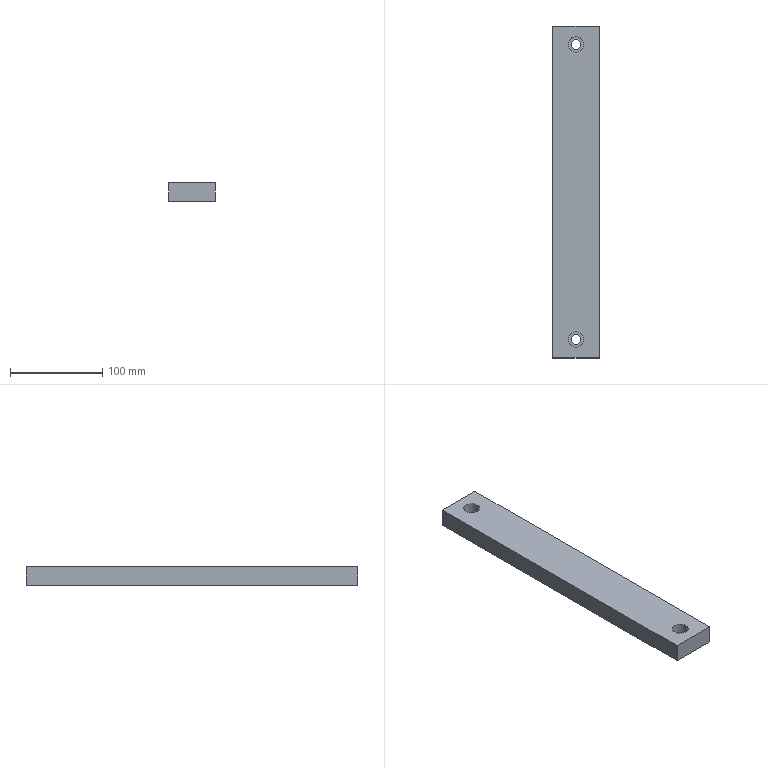Part | STEP file | 200 mesh_id1998 | 1 solid | 12 faces | box 50 x 360 x 20 mm | volume 353388 mm3 | plane 8 | cylinder 4 | commonest cylinder face diameters 10.7 x2 17 x2
STEP:
#1=CARTESIAN_POINT('',(-16927.534,-4180.269,185.258));
#2=VERTEX_POINT('',#1);
#3=CARTESIAN_POINT('',(-16932.884,-4180.269,185.258));
#4=DIRECTION('',(0.,0.,1.));
#5=DIRECTION('',(1.,0.,0.));
#6=AXIS2_PLACEMENT_3D('',#3,#4,#5);
#7=CIRCLE('',#6,5.35);
#8=EDGE_CURVE('',#2,#2,#7,.T.);
#9=ORIENTED_EDGE('',*,*,#8,.F.);
#10=EDGE_LOOP('',(#9));
#11=FACE_BOUND('',#10,.T.);
#12=CARTESIAN_POINT('',(-16924.384,-4180.269,185.258));
#13=VERTEX_POINT('',#12);
#14=CARTESIAN_POINT('',(-16932.884,-4180.269,185.258));
#15=DIRECTION('',(0.,0.,1.));
#16=DIRECTION('',(1.,0.,0.));
#17=AXIS2_PLACEMENT_3D('',#14,#15,#16);
#18=CIRCLE('',#17,8.5);
#19=EDGE_CURVE('',#13,#13,#18,.T.);
#20=ORIENTED_EDGE('',*,*,#19,.T.);
#21=EDGE_LOOP('',(#20));
#22=FACE_BOUND('',#21,.T.);
#23=CARTESIAN_POINT('',(-16932.884,-4180.269,185.258));
#24=DIRECTION('',(0.,0.,-1.));
#25=DIRECTION('',(1.,0.,0.));
#26=AXIS2_PLACEMENT_3D('',#23,#24,#25);
#27=PLANE('',#26);
#28=ADVANCED_FACE('',(#11,#22),#27,.F.);
#29=ORIENTED_EDGE('',*,*,#19,.F.);
#30=EDGE_LOOP('',(#29));
#31=FACE_BOUND('',#30,.T.);
#32=CARTESIAN_POINT('',(-16924.384,-4180.269,196.258));
#33=VERTEX_POINT('',#32);
#34=CARTESIAN_POINT('',(-16932.884,-4180.269,196.258));
#35=DIRECTION('',(0.,0.,-1.));
#36=DIRECTION('',(1.,0.,0.));
#37=AXIS2_PLACEMENT_3D('',#34,#35,#36);
#38=CIRCLE('',#37,8.5);
#39=EDGE_CURVE('',#33,#33,#38,.T.);
#40=ORIENTED_EDGE('',*,*,#39,.F.);
#41=EDGE_LOOP('',(#40));
#42=FACE_BOUND('',#41,.T.);
#43=CARTESIAN_POINT('',(-16932.884,-4180.269,196.258));
#44=DIRECTION('',(0.,0.,-1.));
#45=DIRECTION('',(1.,0.,0.));
#46=AXIS2_PLACEMENT_3D('',#43,#44,#45);
#47=CYLINDRICAL_SURFACE('',#46,8.5);
#48=ADVANCED_FACE('',(#31,#42),#47,.F.);
#49=ORIENTED_EDGE('',*,*,#8,.T.);
#50=EDGE_LOOP('',(#49));
#51=FACE_BOUND('',#50,.T.);
#52=CARTESIAN_POINT('',(-16938.234,-4180.269,176.258));
#53=VERTEX_POINT('',#52);
#54=CARTESIAN_POINT('',(-16932.884,-4180.269,176.258));
#55=DIRECTION('',(0.,0.,1.));
#56=DIRECTION('',(-1.,0.,0.));
#57=AXIS2_PLACEMENT_3D('',#54,#55,#56);
#58=CIRCLE('',#57,5.35);
#59=EDGE_CURVE('',#53,#53,#58,.T.);
#60=ORIENTED_EDGE('',*,*,#59,.F.);
#61=EDGE_LOOP('',(#60));
#62=FACE_BOUND('',#61,.T.);
#63=CARTESIAN_POINT('',(-16932.884,-4180.269,65.92));
#64=DIRECTION('',(0.,0.,-1.));
#65=DIRECTION('',(1.,0.,0.));
#66=AXIS2_PLACEMENT_3D('',#63,#64,#65);
#67=CYLINDRICAL_SURFACE('',#66,5.35);
#68=ADVANCED_FACE('',(#51,#62),#67,.F.);
#69=CARTESIAN_POINT('',(-16927.534,-3860.269,185.258));
#70=VERTEX_POINT('',#69);
#71=CARTESIAN_POINT('',(-16932.884,-3860.269,185.258));
#72=DIRECTION('',(0.,0.,1.));
#73=DIRECTION('',(1.,0.,0.));
#74=AXIS2_PLACEMENT_3D('',#71,#72,#73);
#75=CIRCLE('',#74,5.35);
#76=EDGE_CURVE('',#70,#70,#75,.T.);
#77=ORIENTED_EDGE('',*,*,#76,.F.);
#78=EDGE_LOOP('',(#77));
#79=FACE_BOUND('',#78,.T.);
#80=CARTESIAN_POINT('',(-16924.384,-3860.269,185.258));
#81=VERTEX_POINT('',#80);
#82=CARTESIAN_POINT('',(-16932.884,-3860.269,185.258));
#83=DIRECTION('',(0.,0.,1.));
#84=DIRECTION('',(1.,0.,0.));
#85=AXIS2_PLACEMENT_3D('',#82,#83,#84);
#86=CIRCLE('',#85,8.5);
#87=EDGE_CURVE('',#81,#81,#86,.T.);
#88=ORIENTED_EDGE('',*,*,#87,.T.);
#89=EDGE_LOOP('',(#88));
#90=FACE_BOUND('',#89,.T.);
#91=CARTESIAN_POINT('',(-16932.884,-3860.269,185.258));
#92=DIRECTION('',(0.,0.,-1.));
#93=DIRECTION('',(1.,0.,0.));
#94=AXIS2_PLACEMENT_3D('',#91,#92,#93);
#95=PLANE('',#94);
#96=ADVANCED_FACE('',(#79,#90),#95,.F.);
#97=CARTESIAN_POINT('',(-16957.884,-4200.269,196.258));
#98=VERTEX_POINT('',#97);
#99=CARTESIAN_POINT('',(-16957.884,-4200.269,176.258));
#100=VERTEX_POINT('',#99);
#101=CARTESIAN_POINT('',(-16957.884,-4200.269,176.258));
#102=DIRECTION('',(0.,0.,-1.));
#103=VECTOR('',#102,1.);
#104=LINE('',#101,#103);
#105=EDGE_CURVE('',#98,#100,#104,.T.);
#106=ORIENTED_EDGE('',*,*,#105,.T.);
#107=CARTESIAN_POINT('',(-16907.884,-4200.269,176.258));
#108=VERTEX_POINT('',#107);
#109=CARTESIAN_POINT('',(-16897.884,-4200.269,176.258));
#110=DIRECTION('',(1.,0.,0.));
#111=VECTOR('',#110,1.);
#112=LINE('',#109,#111);
#113=EDGE_CURVE('',#100,#108,#112,.T.);
#114=ORIENTED_EDGE('',*,*,#113,.T.);
#115=CARTESIAN_POINT('',(-16907.884,-4200.269,196.258));
#116=VERTEX_POINT('',#115);
#117=CARTESIAN_POINT('',(-16907.884,-4200.269,176.258));
#118=DIRECTION('',(0.,0.,-1.));
#119=VECTOR('',#118,1.);
#120=LINE('',#117,#119);
#121=EDGE_CURVE('',#116,#108,#120,.T.);
#122=ORIENTED_EDGE('',*,*,#121,.F.);
#123=CARTESIAN_POINT('',(-16897.884,-4200.269,196.258));
#124=DIRECTION('',(1.,0.,0.));
#125=VECTOR('',#124,1.);
#126=LINE('',#123,#125);
#127=EDGE_CURVE('',#98,#116,#126,.T.);
#128=ORIENTED_EDGE('',*,*,#127,.F.);
#129=EDGE_LOOP('',(#106,#114,#122,#128));
#130=FACE_OUTER_BOUND('',#129,.T.);
#131=CARTESIAN_POINT('',(-16897.884,-4200.269,176.258));
#132=DIRECTION('',(0.,1.,0.));
#133=DIRECTION('',(0.,0.,1.));
#134=AXIS2_PLACEMENT_3D('',#131,#132,#133);
#135=PLANE('',#134);
#136=ADVANCED_FACE('',(#130),#135,.F.);
#137=ORIENTED_EDGE('',*,*,#121,.T.);
#138=CARTESIAN_POINT('',(-16907.884,-3840.269,176.258));
#139=VERTEX_POINT('',#138);
#140=CARTESIAN_POINT('',(-16907.884,-3830.269,176.258));
#141=DIRECTION('',(0.,1.,0.));
#142=VECTOR('',#141,1.);
#143=LINE('',#140,#142);
#144=EDGE_CURVE('',#108,#139,#143,.T.);
#145=ORIENTED_EDGE('',*,*,#144,.T.);
#146=CARTESIAN_POINT('',(-16907.884,-3840.269,196.258));
#147=VERTEX_POINT('',#146);
#148=CARTESIAN_POINT('',(-16907.884,-3840.269,196.258));
#149=DIRECTION('',(0.,0.,1.));
#150=VECTOR('',#149,1.);
#151=LINE('',#148,#150);
#152=EDGE_CURVE('',#139,#147,#151,.T.);
#153=ORIENTED_EDGE('',*,*,#152,.T.);
#154=CARTESIAN_POINT('',(-16907.884,-4210.269,196.258));
#155=DIRECTION('',(0.,-1.,0.));
#156=VECTOR('',#155,1.);
#157=LINE('',#154,#156);
#158=EDGE_CURVE('',#147,#116,#157,.T.);
#159=ORIENTED_EDGE('',*,*,#158,.T.);
#160=EDGE_LOOP('',(#137,#145,#153,#159));
#161=FACE_OUTER_BOUND('',#160,.T.);
#162=CARTESIAN_POINT('',(-16907.884,-4180.269,126.258));
#163=DIRECTION('',(-1.,0.,0.));
#164=DIRECTION('',(0.,0.,-1.));
#165=AXIS2_PLACEMENT_3D('',#162,#163,#164);
#166=PLANE('',#165);
#167=ADVANCED_FACE('',(#161),#166,.F.);
#168=CARTESIAN_POINT('',(-16957.884,-3840.269,176.258));
#169=VERTEX_POINT('',#168);
#170=CARTESIAN_POINT('',(-16957.884,-3840.269,196.258));
#171=VERTEX_POINT('',#170);
#172=CARTESIAN_POINT('',(-16957.884,-3840.269,196.258));
#173=DIRECTION('',(0.,0.,1.));
#174=VECTOR('',#173,1.);
#175=LINE('',#172,#174);
#176=EDGE_CURVE('',#169,#171,#175,.T.);
#177=ORIENTED_EDGE('',*,*,#176,.T.);
#178=CARTESIAN_POINT('',(-16897.884,-3840.269,196.258));
#179=DIRECTION('',(1.,0.,0.));
#180=VECTOR('',#179,1.);
#181=LINE('',#178,#180);
#182=EDGE_CURVE('',#171,#147,#181,.T.);
#183=ORIENTED_EDGE('',*,*,#182,.T.);
#184=ORIENTED_EDGE('',*,*,#152,.F.);
#185=CARTESIAN_POINT('',(-16897.884,-3840.269,176.258));
#186=DIRECTION('',(1.,0.,0.));
#187=VECTOR('',#186,1.);
#188=LINE('',#185,#187);
#189=EDGE_CURVE('',#169,#139,#188,.T.);
#190=ORIENTED_EDGE('',*,*,#189,.F.);
#191=EDGE_LOOP('',(#177,#183,#184,#190));
#192=FACE_OUTER_BOUND('',#191,.T.);
#193=CARTESIAN_POINT('',(-16897.884,-3840.269,196.258));
#194=DIRECTION('',(0.,-1.,0.));
#195=DIRECTION('',(0.,0.,-1.));
#196=AXIS2_PLACEMENT_3D('',#193,#194,#195);
#197=PLANE('',#196);
#198=ADVANCED_FACE('',(#192),#197,.F.);
#199=CARTESIAN_POINT('',(-16957.884,-3830.269,176.258));
#200=DIRECTION('',(0.,1.,0.));
#201=VECTOR('',#200,1.);
#202=LINE('',#199,#201);
#203=EDGE_CURVE('',#100,#169,#202,.T.);
#204=ORIENTED_EDGE('',*,*,#203,.F.);
#205=ORIENTED_EDGE('',*,*,#105,.F.);
#206=CARTESIAN_POINT('',(-16957.884,-4210.269,196.258));
#207=DIRECTION('',(0.,-1.,0.));
#208=VECTOR('',#207,1.);
#209=LINE('',#206,#208);
#210=EDGE_CURVE('',#171,#98,#209,.T.);
#211=ORIENTED_EDGE('',*,*,#210,.F.);
#212=ORIENTED_EDGE('',*,*,#176,.F.);
#213=EDGE_LOOP('',(#204,#205,#211,#212));
#214=FACE_OUTER_BOUND('',#213,.T.);
#215=CARTESIAN_POINT('',(-16957.884,0.,15.));
#216=DIRECTION('',(1.,0.,0.));
#217=DIRECTION('',(0.,0.,1.));
#218=AXIS2_PLACEMENT_3D('',#215,#216,#217);
#219=PLANE('',#218);
#220=ADVANCED_FACE('',(#214),#219,.F.);
#221=ORIENTED_EDGE('',*,*,#87,.F.);
#222=EDGE_LOOP('',(#221));
#223=FACE_BOUND('',#222,.T.);
#224=CARTESIAN_POINT('',(-16924.384,-3860.269,196.258));
#225=VERTEX_POINT('',#224);
#226=CARTESIAN_POINT('',(-16932.884,-3860.269,196.258));
#227=DIRECTION('',(0.,0.,-1.));
#228=DIRECTION('',(1.,0.,0.));
#229=AXIS2_PLACEMENT_3D('',#226,#227,#228);
#230=CIRCLE('',#229,8.5);
#231=EDGE_CURVE('',#225,#225,#230,.T.);
#232=ORIENTED_EDGE('',*,*,#231,.F.);
#233=EDGE_LOOP('',(#232));
#234=FACE_BOUND('',#233,.T.);
#235=CARTESIAN_POINT('',(-16932.884,-3860.269,196.258));
#236=DIRECTION('',(0.,0.,-1.));
#237=DIRECTION('',(1.,0.,0.));
#238=AXIS2_PLACEMENT_3D('',#235,#236,#237);
#239=CYLINDRICAL_SURFACE('',#238,8.5);
#240=ADVANCED_FACE('',(#223,#234),#239,.F.);
#241=ORIENTED_EDGE('',*,*,#182,.F.);
#242=ORIENTED_EDGE('',*,*,#210,.T.);
#243=ORIENTED_EDGE('',*,*,#127,.T.);
#244=ORIENTED_EDGE('',*,*,#158,.F.);
#245=EDGE_LOOP('',(#241,#242,#243,#244));
#246=FACE_BOUND('',#245,.T.);
#247=ORIENTED_EDGE('',*,*,#39,.T.);
#248=EDGE_LOOP('',(#247));
#249=FACE_BOUND('',#248,.T.);
#250=ORIENTED_EDGE('',*,*,#231,.T.);
#251=EDGE_LOOP('',(#250));
#252=FACE_BOUND('',#251,.T.);
#253=CARTESIAN_POINT('',(-16897.884,-4210.269,196.258));
#254=DIRECTION('',(0.,0.,-1.));
#255=DIRECTION('',(1.,0.,0.));
#256=AXIS2_PLACEMENT_3D('',#253,#254,#255);
#257=PLANE('',#256);
#258=ADVANCED_FACE('',(#246,#249,#252),#257,.F.);
#259=ORIENTED_EDGE('',*,*,#76,.T.);
#260=EDGE_LOOP('',(#259));
#261=FACE_BOUND('',#260,.T.);
#262=CARTESIAN_POINT('',(-16938.234,-3860.269,176.258));
#263=VERTEX_POINT('',#262);
#264=CARTESIAN_POINT('',(-16932.884,-3860.269,176.258));
#265=DIRECTION('',(0.,0.,1.));
#266=DIRECTION('',(-1.,0.,0.));
#267=AXIS2_PLACEMENT_3D('',#264,#265,#266);
#268=CIRCLE('',#267,5.35);
#269=EDGE_CURVE('',#263,#263,#268,.T.);
#270=ORIENTED_EDGE('',*,*,#269,.F.);
#271=EDGE_LOOP('',(#270));
#272=FACE_BOUND('',#271,.T.);
#273=CARTESIAN_POINT('',(-16932.884,-3860.269,65.92));
#274=DIRECTION('',(0.,0.,-1.));
#275=DIRECTION('',(1.,0.,0.));
#276=AXIS2_PLACEMENT_3D('',#273,#274,#275);
#277=CYLINDRICAL_SURFACE('',#276,5.35);
#278=ADVANCED_FACE('',(#261,#272),#277,.F.);
#279=ORIENTED_EDGE('',*,*,#113,.F.);
#280=ORIENTED_EDGE('',*,*,#203,.T.);
#281=ORIENTED_EDGE('',*,*,#189,.T.);
#282=ORIENTED_EDGE('',*,*,#144,.F.);
#283=EDGE_LOOP('',(#279,#280,#281,#282));
#284=FACE_BOUND('',#283,.T.);
#285=ORIENTED_EDGE('',*,*,#59,.T.);
#286=EDGE_LOOP('',(#285));
#287=FACE_BOUND('',#286,.T.);
#288=ORIENTED_EDGE('',*,*,#269,.T.);
#289=EDGE_LOOP('',(#288));
#290=FACE_BOUND('',#289,.T.);
#291=CARTESIAN_POINT('',(-16897.884,-3830.269,176.258));
#292=DIRECTION('',(0.,0.,1.));
#293=DIRECTION('',(-1.,0.,0.));
#294=AXIS2_PLACEMENT_3D('',#291,#292,#293);
#295=PLANE('',#294);
#296=ADVANCED_FACE('',(#284,#287,#290),#295,.F.);
#297=CLOSED_SHELL('',(#28,#48,#68,#96,#136,#167,#198,#220,#240,#258,#278,#296));
#298=MANIFOLD_SOLID_BREP('',#297);
#299=(LENGTH_UNIT()NAMED_UNIT(*)SI_UNIT(.MILLI.,.METRE.));
#300=UNCERTAINTY_MEASURE_WITH_UNIT(LENGTH_MEASURE(0.00002),#299,'','');
#301=(NAMED_UNIT(*)PLANE_ANGLE_UNIT()SI_UNIT($,.RADIAN.));
#302=PLANE_ANGLE_MEASURE_WITH_UNIT(PLANE_ANGLE_MEASURE(0.01745),#301);
#303=DIMENSIONAL_EXPONENTS(0.,0.,0.,0.,0.,0.,0.);
#304=(CONVERSION_BASED_UNIT('DEGREE',#302)NAMED_UNIT(#303)PLANE_ANGLE_UNIT());
#305=(NAMED_UNIT(*)SI_UNIT($,.STERADIAN.)SOLID_ANGLE_UNIT());
#306=(GEOMETRIC_REPRESENTATION_CONTEXT(3)GLOBAL_UNCERTAINTY_ASSIGNED_CONTEXT((#300))GLOBAL_UNIT_ASSIGNED_CONTEXT((#299,#304,#305))REPRESENTATION_CONTEXT('',''));
#307=ADVANCED_BREP_SHAPE_REPRESENTATION('',(#298),#306);